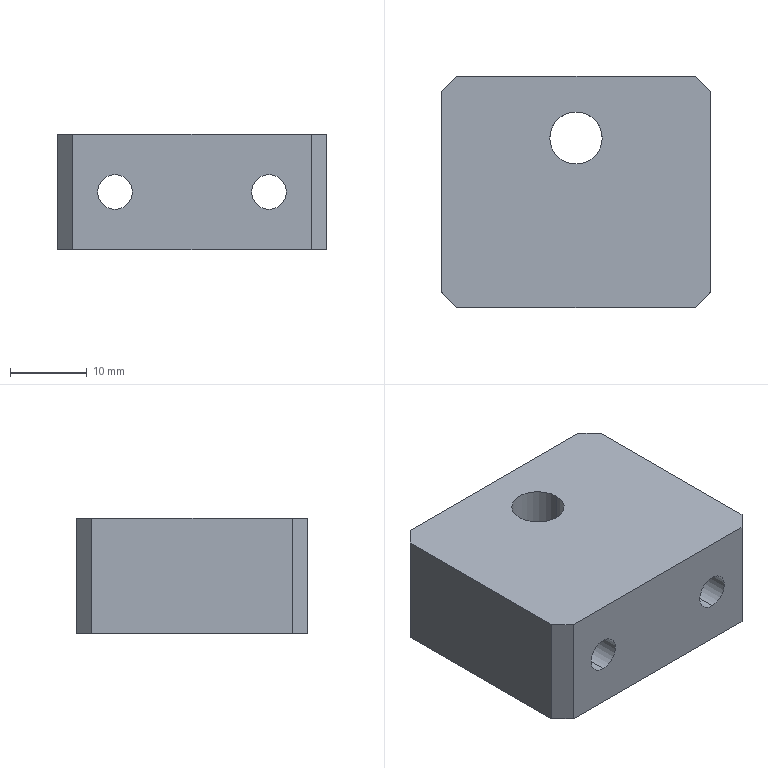Part | SolidWorks | features HoleWzd 2, Chamfer 1, Extrusion 1 | 1 solid | 22 faces | box 35 x 30 x 15 mm | volume 13829 mm3 | plane 12 | cylinder 10 | commonest cylinder face diameters 4.5 x4 8 x4 6.8 x2
STEP:
#1=CARTESIAN_POINT('',(-3.4,7.,0.));
#2=VERTEX_POINT('',#1);
#3=CARTESIAN_POINT('',(3.4,7.,0.));
#4=VERTEX_POINT('',#3);
#5=CARTESIAN_POINT('',(0.,7.,0.));
#6=DIRECTION('',(0.,0.,1.));
#7=DIRECTION('',(1.,0.,0.));
#8=AXIS2_PLACEMENT_3D('',#5,#6,#7);
#9=CIRCLE('',#8,3.4);
#10=EDGE_CURVE('',#2,#4,#9,.T.);
#11=ORIENTED_EDGE('',*,*,#10,.F.);
#12=CARTESIAN_POINT('',(-3.4,7.,15.));
#13=VERTEX_POINT('',#12);
#14=CARTESIAN_POINT('',(-3.4,7.,15.));
#15=DIRECTION('',(0.,0.,1.));
#16=VECTOR('',#15,1000.);
#17=LINE('',#14,#16);
#18=EDGE_CURVE('',#2,#13,#17,.T.);
#19=ORIENTED_EDGE('',*,*,#18,.T.);
#20=CARTESIAN_POINT('',(3.4,7.,15.));
#21=VERTEX_POINT('',#20);
#22=CARTESIAN_POINT('',(0.,7.,15.));
#23=DIRECTION('',(0.,0.,1.));
#24=DIRECTION('',(1.,0.,0.));
#25=AXIS2_PLACEMENT_3D('',#22,#23,#24);
#26=CIRCLE('',#25,3.4);
#27=EDGE_CURVE('',#13,#21,#26,.T.);
#28=ORIENTED_EDGE('',*,*,#27,.T.);
#29=CARTESIAN_POINT('',(3.4,7.,15.));
#30=DIRECTION('',(0.,0.,1.));
#31=VECTOR('',#30,1000.);
#32=LINE('',#29,#31);
#33=EDGE_CURVE('',#4,#21,#32,.T.);
#34=ORIENTED_EDGE('',*,*,#33,.F.);
#35=EDGE_LOOP('',(#11,#19,#28,#34));
#36=FACE_OUTER_BOUND('',#35,.T.);
#37=CARTESIAN_POINT('',(0.,7.,15.));
#38=DIRECTION('',(0.,0.,1.));
#39=DIRECTION('',(1.,0.,0.));
#40=AXIS2_PLACEMENT_3D('',#37,#38,#39);
#41=CYLINDRICAL_SURFACE('',#40,3.4);
#42=ADVANCED_FACE('',(#36),#41,.F.);
#43=CARTESIAN_POINT('',(-10.,10.6,3.5));
#44=VERTEX_POINT('',#43);
#45=CARTESIAN_POINT('',(-10.,10.6,11.5));
#46=VERTEX_POINT('',#45);
#47=CARTESIAN_POINT('',(-10.,10.6,7.5));
#48=DIRECTION('',(0.,1.,0.));
#49=DIRECTION('',(0.,0.,1.));
#50=AXIS2_PLACEMENT_3D('',#47,#48,#49);
#51=CIRCLE('',#50,4.);
#52=EDGE_CURVE('',#44,#46,#51,.T.);
#53=ORIENTED_EDGE('',*,*,#52,.F.);
#54=CARTESIAN_POINT('',(-10.,15.,3.5));
#55=VERTEX_POINT('',#54);
#56=CARTESIAN_POINT('',(-10.,15.,3.5));
#57=DIRECTION('',(0.,1.,0.));
#58=VECTOR('',#57,1000.);
#59=LINE('',#56,#58);
#60=EDGE_CURVE('',#44,#55,#59,.T.);
#61=ORIENTED_EDGE('',*,*,#60,.T.);
#62=CARTESIAN_POINT('',(-10.,15.,11.5));
#63=VERTEX_POINT('',#62);
#64=CARTESIAN_POINT('',(-10.,15.,7.5));
#65=DIRECTION('',(0.,1.,0.));
#66=DIRECTION('',(0.,0.,1.));
#67=AXIS2_PLACEMENT_3D('',#64,#65,#66);
#68=CIRCLE('',#67,4.);
#69=EDGE_CURVE('',#55,#63,#68,.T.);
#70=ORIENTED_EDGE('',*,*,#69,.T.);
#71=CARTESIAN_POINT('',(-10.,15.,11.5));
#72=DIRECTION('',(0.,1.,0.));
#73=VECTOR('',#72,1000.);
#74=LINE('',#71,#73);
#75=EDGE_CURVE('',#46,#63,#74,.T.);
#76=ORIENTED_EDGE('',*,*,#75,.F.);
#77=EDGE_LOOP('',(#53,#61,#70,#76));
#78=FACE_OUTER_BOUND('',#77,.T.);
#79=CARTESIAN_POINT('',(-10.,15.,7.5));
#80=DIRECTION('',(0.,1.,0.));
#81=DIRECTION('',(0.,0.,1.));
#82=AXIS2_PLACEMENT_3D('',#79,#80,#81);
#83=CYLINDRICAL_SURFACE('',#82,4.);
#84=ADVANCED_FACE('',(#78),#83,.F.);
#85=CARTESIAN_POINT('',(-10.,-15.,5.25));
#86=VERTEX_POINT('',#85);
#87=CARTESIAN_POINT('',(-10.,-15.,9.75));
#88=VERTEX_POINT('',#87);
#89=CARTESIAN_POINT('',(-10.,-15.,7.5));
#90=DIRECTION('',(0.,1.,0.));
#91=DIRECTION('',(0.,0.,1.));
#92=AXIS2_PLACEMENT_3D('',#89,#90,#91);
#93=CIRCLE('',#92,2.25);
#94=EDGE_CURVE('',#86,#88,#93,.T.);
#95=ORIENTED_EDGE('',*,*,#94,.F.);
#96=CARTESIAN_POINT('',(-10.,10.6,5.25));
#97=VERTEX_POINT('',#96);
#98=CARTESIAN_POINT('',(-10.,15.,5.25));
#99=DIRECTION('',(0.,1.,0.));
#100=VECTOR('',#99,1000.);
#101=LINE('',#98,#100);
#102=EDGE_CURVE('',#86,#97,#101,.T.);
#103=ORIENTED_EDGE('',*,*,#102,.T.);
#104=CARTESIAN_POINT('',(-10.,10.6,9.75));
#105=VERTEX_POINT('',#104);
#106=CARTESIAN_POINT('',(-10.,10.6,7.5));
#107=DIRECTION('',(0.,1.,0.));
#108=DIRECTION('',(0.,0.,1.));
#109=AXIS2_PLACEMENT_3D('',#106,#107,#108);
#110=CIRCLE('',#109,2.25);
#111=EDGE_CURVE('',#97,#105,#110,.T.);
#112=ORIENTED_EDGE('',*,*,#111,.T.);
#113=CARTESIAN_POINT('',(-10.,15.,9.75));
#114=DIRECTION('',(0.,1.,0.));
#115=VECTOR('',#114,1000.);
#116=LINE('',#113,#115);
#117=EDGE_CURVE('',#88,#105,#116,.T.);
#118=ORIENTED_EDGE('',*,*,#117,.F.);
#119=EDGE_LOOP('',(#95,#103,#112,#118));
#120=FACE_OUTER_BOUND('',#119,.T.);
#121=CARTESIAN_POINT('',(-10.,15.,7.5));
#122=DIRECTION('',(0.,1.,0.));
#123=DIRECTION('',(0.,0.,1.));
#124=AXIS2_PLACEMENT_3D('',#121,#122,#123);
#125=CYLINDRICAL_SURFACE('',#124,2.25);
#126=ADVANCED_FACE('',(#120),#125,.F.);
#127=CARTESIAN_POINT('',(10.,10.6,3.5));
#128=VERTEX_POINT('',#127);
#129=CARTESIAN_POINT('',(10.,10.6,11.5));
#130=VERTEX_POINT('',#129);
#131=CARTESIAN_POINT('',(10.,10.6,7.5));
#132=DIRECTION('',(0.,1.,0.));
#133=DIRECTION('',(0.,0.,1.));
#134=AXIS2_PLACEMENT_3D('',#131,#132,#133);
#135=CIRCLE('',#134,4.);
#136=EDGE_CURVE('',#128,#130,#135,.T.);
#137=ORIENTED_EDGE('',*,*,#136,.F.);
#138=CARTESIAN_POINT('',(10.,15.,3.5));
#139=VERTEX_POINT('',#138);
#140=CARTESIAN_POINT('',(10.,15.,3.5));
#141=DIRECTION('',(0.,1.,0.));
#142=VECTOR('',#141,1000.);
#143=LINE('',#140,#142);
#144=EDGE_CURVE('',#128,#139,#143,.T.);
#145=ORIENTED_EDGE('',*,*,#144,.T.);
#146=CARTESIAN_POINT('',(10.,15.,11.5));
#147=VERTEX_POINT('',#146);
#148=CARTESIAN_POINT('',(10.,15.,7.5));
#149=DIRECTION('',(0.,1.,0.));
#150=DIRECTION('',(0.,0.,1.));
#151=AXIS2_PLACEMENT_3D('',#148,#149,#150);
#152=CIRCLE('',#151,4.);
#153=EDGE_CURVE('',#139,#147,#152,.T.);
#154=ORIENTED_EDGE('',*,*,#153,.T.);
#155=CARTESIAN_POINT('',(10.,15.,11.5));
#156=DIRECTION('',(0.,1.,0.));
#157=VECTOR('',#156,1000.);
#158=LINE('',#155,#157);
#159=EDGE_CURVE('',#130,#147,#158,.T.);
#160=ORIENTED_EDGE('',*,*,#159,.F.);
#161=EDGE_LOOP('',(#137,#145,#154,#160));
#162=FACE_OUTER_BOUND('',#161,.T.);
#163=CARTESIAN_POINT('',(10.,15.,7.5));
#164=DIRECTION('',(0.,1.,0.));
#165=DIRECTION('',(0.,0.,1.));
#166=AXIS2_PLACEMENT_3D('',#163,#164,#165);
#167=CYLINDRICAL_SURFACE('',#166,4.);
#168=ADVANCED_FACE('',(#162),#167,.F.);
#169=CARTESIAN_POINT('',(10.,-15.,5.25));
#170=VERTEX_POINT('',#169);
#171=CARTESIAN_POINT('',(10.,-15.,9.75));
#172=VERTEX_POINT('',#171);
#173=CARTESIAN_POINT('',(10.,-15.,7.5));
#174=DIRECTION('',(0.,1.,0.));
#175=DIRECTION('',(0.,0.,1.));
#176=AXIS2_PLACEMENT_3D('',#173,#174,#175);
#177=CIRCLE('',#176,2.25);
#178=EDGE_CURVE('',#170,#172,#177,.T.);
#179=ORIENTED_EDGE('',*,*,#178,.F.);
#180=CARTESIAN_POINT('',(10.,10.6,5.25));
#181=VERTEX_POINT('',#180);
#182=CARTESIAN_POINT('',(10.,15.,5.25));
#183=DIRECTION('',(0.,1.,0.));
#184=VECTOR('',#183,1000.);
#185=LINE('',#182,#184);
#186=EDGE_CURVE('',#170,#181,#185,.T.);
#187=ORIENTED_EDGE('',*,*,#186,.T.);
#188=CARTESIAN_POINT('',(10.,10.6,9.75));
#189=VERTEX_POINT('',#188);
#190=CARTESIAN_POINT('',(10.,10.6,7.5));
#191=DIRECTION('',(0.,1.,0.));
#192=DIRECTION('',(0.,0.,1.));
#193=AXIS2_PLACEMENT_3D('',#190,#191,#192);
#194=CIRCLE('',#193,2.25);
#195=EDGE_CURVE('',#181,#189,#194,.T.);
#196=ORIENTED_EDGE('',*,*,#195,.T.);
#197=CARTESIAN_POINT('',(10.,15.,9.75));
#198=DIRECTION('',(0.,1.,0.));
#199=VECTOR('',#198,1000.);
#200=LINE('',#197,#199);
#201=EDGE_CURVE('',#172,#189,#200,.T.);
#202=ORIENTED_EDGE('',*,*,#201,.F.);
#203=EDGE_LOOP('',(#179,#187,#196,#202));
#204=FACE_OUTER_BOUND('',#203,.T.);
#205=CARTESIAN_POINT('',(10.,15.,7.5));
#206=DIRECTION('',(0.,1.,0.));
#207=DIRECTION('',(0.,0.,1.));
#208=AXIS2_PLACEMENT_3D('',#205,#206,#207);
#209=CYLINDRICAL_SURFACE('',#208,2.25);
#210=ADVANCED_FACE('',(#204),#209,.F.);
#211=CARTESIAN_POINT('',(17.5,-13.,15.));
#212=VERTEX_POINT('',#211);
#213=CARTESIAN_POINT('',(17.5,13.,15.));
#214=VERTEX_POINT('',#213);
#215=CARTESIAN_POINT('',(17.5,15.,15.));
#216=DIRECTION('',(0.,1.,0.));
#217=VECTOR('',#216,1000.);
#218=LINE('',#215,#217);
#219=EDGE_CURVE('',#212,#214,#218,.T.);
#220=ORIENTED_EDGE('',*,*,#219,.F.);
#221=CARTESIAN_POINT('',(17.5,-13.,0.));
#222=VERTEX_POINT('',#221);
#223=CARTESIAN_POINT('',(17.5,-13.,15.));
#224=DIRECTION('',(0.,0.,-1.));
#225=VECTOR('',#224,1000.);
#226=LINE('',#223,#225);
#227=EDGE_CURVE('',#212,#222,#226,.T.);
#228=ORIENTED_EDGE('',*,*,#227,.T.);
#229=CARTESIAN_POINT('',(17.5,13.,0.));
#230=VERTEX_POINT('',#229);
#231=CARTESIAN_POINT('',(17.5,15.,0.));
#232=DIRECTION('',(0.,1.,0.));
#233=VECTOR('',#232,1000.);
#234=LINE('',#231,#233);
#235=EDGE_CURVE('',#222,#230,#234,.T.);
#236=ORIENTED_EDGE('',*,*,#235,.T.);
#237=CARTESIAN_POINT('',(17.5,13.,15.));
#238=DIRECTION('',(0.,0.,1.));
#239=VECTOR('',#238,1000.);
#240=LINE('',#237,#239);
#241=EDGE_CURVE('',#230,#214,#240,.T.);
#242=ORIENTED_EDGE('',*,*,#241,.T.);
#243=EDGE_LOOP('',(#220,#228,#236,#242));
#244=FACE_OUTER_BOUND('',#243,.T.);
#245=CARTESIAN_POINT('',(17.5,15.,15.));
#246=DIRECTION('',(-1.,0.,0.));
#247=DIRECTION('',(0.,-1.,0.));
#248=AXIS2_PLACEMENT_3D('',#245,#246,#247);
#249=PLANE('',#248);
#250=ADVANCED_FACE('',(#244),#249,.F.);
#251=CARTESIAN_POINT('',(-10.,15.,7.5));
#252=DIRECTION('',(0.,1.,0.));
#253=DIRECTION('',(0.,0.,1.));
#254=AXIS2_PLACEMENT_3D('',#251,#252,#253);
#255=CIRCLE('',#254,4.);
#256=EDGE_CURVE('',#63,#55,#255,.T.);
#257=ORIENTED_EDGE('',*,*,#256,.F.);
#258=ORIENTED_EDGE('',*,*,#69,.F.);
#259=EDGE_LOOP('',(#257,#258));
#260=FACE_BOUND('',#259,.T.);
#261=CARTESIAN_POINT('',(10.,15.,7.5));
#262=DIRECTION('',(0.,1.,0.));
#263=DIRECTION('',(0.,0.,1.));
#264=AXIS2_PLACEMENT_3D('',#261,#262,#263);
#265=CIRCLE('',#264,4.);
#266=EDGE_CURVE('',#147,#139,#265,.T.);
#267=ORIENTED_EDGE('',*,*,#266,.F.);
#268=ORIENTED_EDGE('',*,*,#153,.F.);
#269=EDGE_LOOP('',(#267,#268));
#270=FACE_BOUND('',#269,.T.);
#271=CARTESIAN_POINT('',(15.5,15.,15.));
#272=VERTEX_POINT('',#271);
#273=CARTESIAN_POINT('',(-15.5,15.,15.));
#274=VERTEX_POINT('',#273);
#275=CARTESIAN_POINT('',(-17.5,15.,15.));
#276=DIRECTION('',(-1.,0.,0.));
#277=VECTOR('',#276,1000.);
#278=LINE('',#275,#277);
#279=EDGE_CURVE('',#272,#274,#278,.T.);
#280=ORIENTED_EDGE('',*,*,#279,.F.);
#281=CARTESIAN_POINT('',(15.5,15.,0.));
#282=VERTEX_POINT('',#281);
#283=CARTESIAN_POINT('',(15.5,15.,15.));
#284=DIRECTION('',(0.,0.,-1.));
#285=VECTOR('',#284,1000.);
#286=LINE('',#283,#285);
#287=EDGE_CURVE('',#272,#282,#286,.T.);
#288=ORIENTED_EDGE('',*,*,#287,.T.);
#289=CARTESIAN_POINT('',(-15.5,15.,0.));
#290=VERTEX_POINT('',#289);
#291=CARTESIAN_POINT('',(-17.5,15.,0.));
#292=DIRECTION('',(-1.,0.,0.));
#293=VECTOR('',#292,1000.);
#294=LINE('',#291,#293);
#295=EDGE_CURVE('',#282,#290,#294,.T.);
#296=ORIENTED_EDGE('',*,*,#295,.T.);
#297=CARTESIAN_POINT('',(-15.5,15.,15.));
#298=DIRECTION('',(0.,0.,1.));
#299=VECTOR('',#298,1000.);
#300=LINE('',#297,#299);
#301=EDGE_CURVE('',#290,#274,#300,.T.);
#302=ORIENTED_EDGE('',*,*,#301,.T.);
#303=EDGE_LOOP('',(#280,#288,#296,#302));
#304=FACE_OUTER_BOUND('',#303,.T.);
#305=CARTESIAN_POINT('',(-17.5,15.,15.));
#306=DIRECTION('',(0.,-1.,0.));
#307=DIRECTION('',(0.,0.,-1.));
#308=AXIS2_PLACEMENT_3D('',#305,#306,#307);
#309=PLANE('',#308);
#310=ADVANCED_FACE('',(#260,#270,#304),#309,.F.);
#311=CARTESIAN_POINT('',(-17.5,13.,0.));
#312=VERTEX_POINT('',#311);
#313=CARTESIAN_POINT('',(-17.5,-13.,0.));
#314=VERTEX_POINT('',#313);
#315=CARTESIAN_POINT('',(-17.5,15.,0.));
#316=DIRECTION('',(0.,-1.,0.));
#317=VECTOR('',#316,1000.);
#318=LINE('',#315,#317);
#319=EDGE_CURVE('',#312,#314,#318,.T.);
#320=ORIENTED_EDGE('',*,*,#319,.T.);
#321=CARTESIAN_POINT('',(-17.5,-13.,15.));
#322=VERTEX_POINT('',#321);
#323=CARTESIAN_POINT('',(-17.5,-13.,15.));
#324=DIRECTION('',(0.,0.,1.));
#325=VECTOR('',#324,1000.);
#326=LINE('',#323,#325);
#327=EDGE_CURVE('',#314,#322,#326,.T.);
#328=ORIENTED_EDGE('',*,*,#327,.T.);
#329=CARTESIAN_POINT('',(-17.5,13.,15.));
#330=VERTEX_POINT('',#329);
#331=CARTESIAN_POINT('',(-17.5,15.,15.));
#332=DIRECTION('',(0.,-1.,0.));
#333=VECTOR('',#332,1000.);
#334=LINE('',#331,#333);
#335=EDGE_CURVE('',#330,#322,#334,.T.);
#336=ORIENTED_EDGE('',*,*,#335,.F.);
#337=CARTESIAN_POINT('',(-17.5,13.,15.));
#338=DIRECTION('',(0.,0.,-1.));
#339=VECTOR('',#338,1000.);
#340=LINE('',#337,#339);
#341=EDGE_CURVE('',#330,#312,#340,.T.);
#342=ORIENTED_EDGE('',*,*,#341,.T.);
#343=EDGE_LOOP('',(#320,#328,#336,#342));
#344=FACE_OUTER_BOUND('',#343,.T.);
#345=CARTESIAN_POINT('',(-17.5,15.,15.));
#346=DIRECTION('',(1.,0.,0.));
#347=DIRECTION('',(0.,1.,0.));
#348=AXIS2_PLACEMENT_3D('',#345,#346,#347);
#349=PLANE('',#348);
#350=ADVANCED_FACE('',(#344),#349,.F.);
#351=CARTESIAN_POINT('',(-10.,-15.,7.5));
#352=DIRECTION('',(0.,1.,0.));
#353=DIRECTION('',(0.,0.,1.));
#354=AXIS2_PLACEMENT_3D('',#351,#352,#353);
#355=CIRCLE('',#354,2.25);
#356=EDGE_CURVE('',#88,#86,#355,.T.);
#357=ORIENTED_EDGE('',*,*,#356,.T.);
#358=ORIENTED_EDGE('',*,*,#94,.T.);
#359=EDGE_LOOP('',(#357,#358));
#360=FACE_BOUND('',#359,.T.);
#361=CARTESIAN_POINT('',(10.,-15.,7.5));
#362=DIRECTION('',(0.,1.,0.));
#363=DIRECTION('',(0.,0.,1.));
#364=AXIS2_PLACEMENT_3D('',#361,#362,#363);
#365=CIRCLE('',#364,2.25);
#366=EDGE_CURVE('',#172,#170,#365,.T.);
#367=ORIENTED_EDGE('',*,*,#366,.T.);
#368=ORIENTED_EDGE('',*,*,#178,.T.);
#369=EDGE_LOOP('',(#367,#368));
#370=FACE_BOUND('',#369,.T.);
#371=CARTESIAN_POINT('',(-15.5,-15.,15.));
#372=VERTEX_POINT('',#371);
#373=CARTESIAN_POINT('',(15.5,-15.,15.));
#374=VERTEX_POINT('',#373);
#375=CARTESIAN_POINT('',(-17.5,-15.,15.));
#376=DIRECTION('',(1.,0.,0.));
#377=VECTOR('',#376,1000.);
#378=LINE('',#375,#377);
#379=EDGE_CURVE('',#372,#374,#378,.T.);
#380=ORIENTED_EDGE('',*,*,#379,.F.);
#381=CARTESIAN_POINT('',(-15.5,-15.,0.));
#382=VERTEX_POINT('',#381);
#383=CARTESIAN_POINT('',(-15.5,-15.,15.));
#384=DIRECTION('',(0.,0.,-1.));
#385=VECTOR('',#384,1000.);
#386=LINE('',#383,#385);
#387=EDGE_CURVE('',#372,#382,#386,.T.);
#388=ORIENTED_EDGE('',*,*,#387,.T.);
#389=CARTESIAN_POINT('',(15.5,-15.,0.));
#390=VERTEX_POINT('',#389);
#391=CARTESIAN_POINT('',(-17.5,-15.,0.));
#392=DIRECTION('',(1.,0.,0.));
#393=VECTOR('',#392,1000.);
#394=LINE('',#391,#393);
#395=EDGE_CURVE('',#382,#390,#394,.T.);
#396=ORIENTED_EDGE('',*,*,#395,.T.);
#397=CARTESIAN_POINT('',(15.5,-15.,15.));
#398=DIRECTION('',(0.,0.,1.));
#399=VECTOR('',#398,1000.);
#400=LINE('',#397,#399);
#401=EDGE_CURVE('',#390,#374,#400,.T.);
#402=ORIENTED_EDGE('',*,*,#401,.T.);
#403=EDGE_LOOP('',(#380,#388,#396,#402));
#404=FACE_OUTER_BOUND('',#403,.T.);
#405=CARTESIAN_POINT('',(-17.5,-15.,15.));
#406=DIRECTION('',(0.,1.,0.));
#407=DIRECTION('',(0.,0.,1.));
#408=AXIS2_PLACEMENT_3D('',#405,#406,#407);
#409=PLANE('',#408);
#410=ADVANCED_FACE('',(#360,#370,#404),#409,.F.);
#411=CARTESIAN_POINT('',(0.,7.,15.));
#412=DIRECTION('',(0.,0.,1.));
#413=DIRECTION('',(1.,0.,0.));
#414=AXIS2_PLACEMENT_3D('',#411,#412,#413);
#415=CIRCLE('',#414,3.4);
#416=EDGE_CURVE('',#21,#13,#415,.T.);
#417=ORIENTED_EDGE('',*,*,#416,.F.);
#418=ORIENTED_EDGE('',*,*,#27,.F.);
#419=EDGE_LOOP('',(#417,#418));
#420=FACE_BOUND('',#419,.T.);
#421=ORIENTED_EDGE('',*,*,#335,.T.);
#422=CARTESIAN_POINT('',(-15.25,-15.25,15.));
#423=DIRECTION('',(0.7071,-0.7071,0.));
#424=VECTOR('',#423,1000.);
#425=LINE('',#422,#424);
#426=EDGE_CURVE('',#322,#372,#425,.T.);
#427=ORIENTED_EDGE('',*,*,#426,.T.);
#428=ORIENTED_EDGE('',*,*,#379,.T.);
#429=CARTESIAN_POINT('',(15.25,-15.25,15.));
#430=DIRECTION('',(0.7071,0.7071,0.));
#431=VECTOR('',#430,1000.);
#432=LINE('',#429,#431);
#433=EDGE_CURVE('',#374,#212,#432,.T.);
#434=ORIENTED_EDGE('',*,*,#433,.T.);
#435=ORIENTED_EDGE('',*,*,#219,.T.);
#436=CARTESIAN_POINT('',(15.25,15.25,15.));
#437=DIRECTION('',(-0.7071,0.7071,0.));
#438=VECTOR('',#437,1000.);
#439=LINE('',#436,#438);
#440=EDGE_CURVE('',#214,#272,#439,.T.);
#441=ORIENTED_EDGE('',*,*,#440,.T.);
#442=ORIENTED_EDGE('',*,*,#279,.T.);
#443=CARTESIAN_POINT('',(-15.25,15.25,15.));
#444=DIRECTION('',(-0.7071,-0.7071,0.));
#445=VECTOR('',#444,1000.);
#446=LINE('',#443,#445);
#447=EDGE_CURVE('',#274,#330,#446,.T.);
#448=ORIENTED_EDGE('',*,*,#447,.T.);
#449=EDGE_LOOP('',(#421,#427,#428,#434,#435,#441,#442,#448));
#450=FACE_OUTER_BOUND('',#449,.T.);
#451=CARTESIAN_POINT('',(0.,0.,15.));
#452=DIRECTION('',(0.,0.,1.));
#453=DIRECTION('',(1.,0.,0.));
#454=AXIS2_PLACEMENT_3D('',#451,#452,#453);
#455=PLANE('',#454);
#456=ADVANCED_FACE('',(#420,#450),#455,.T.);
#457=CARTESIAN_POINT('',(0.,7.,0.));
#458=DIRECTION('',(0.,0.,1.));
#459=DIRECTION('',(1.,0.,0.));
#460=AXIS2_PLACEMENT_3D('',#457,#458,#459);
#461=CIRCLE('',#460,3.4);
#462=EDGE_CURVE('',#4,#2,#461,.T.);
#463=ORIENTED_EDGE('',*,*,#462,.T.);
#464=ORIENTED_EDGE('',*,*,#10,.T.);
#465=EDGE_LOOP('',(#463,#464));
#466=FACE_BOUND('',#465,.T.);
#467=ORIENTED_EDGE('',*,*,#395,.F.);
#468=CARTESIAN_POINT('',(-15.5,-15.,0.));
#469=DIRECTION('',(-0.7071,0.7071,0.));
#470=VECTOR('',#469,1000.);
#471=LINE('',#468,#470);
#472=EDGE_CURVE('',#382,#314,#471,.T.);
#473=ORIENTED_EDGE('',*,*,#472,.T.);
#474=ORIENTED_EDGE('',*,*,#319,.F.);
#475=CARTESIAN_POINT('',(-17.5,13.,0.));
#476=DIRECTION('',(0.7071,0.7071,0.));
#477=VECTOR('',#476,1000.);
#478=LINE('',#475,#477);
#479=EDGE_CURVE('',#312,#290,#478,.T.);
#480=ORIENTED_EDGE('',*,*,#479,.T.);
#481=ORIENTED_EDGE('',*,*,#295,.F.);
#482=CARTESIAN_POINT('',(15.5,15.,0.));
#483=DIRECTION('',(0.7071,-0.7071,0.));
#484=VECTOR('',#483,1000.);
#485=LINE('',#482,#484);
#486=EDGE_CURVE('',#282,#230,#485,.T.);
#487=ORIENTED_EDGE('',*,*,#486,.T.);
#488=ORIENTED_EDGE('',*,*,#235,.F.);
#489=CARTESIAN_POINT('',(17.5,-13.,0.));
#490=DIRECTION('',(-0.7071,-0.7071,0.));
#491=VECTOR('',#490,1000.);
#492=LINE('',#489,#491);
#493=EDGE_CURVE('',#222,#390,#492,.T.);
#494=ORIENTED_EDGE('',*,*,#493,.T.);
#495=EDGE_LOOP('',(#467,#473,#474,#480,#481,#487,#488,#494));
#496=FACE_OUTER_BOUND('',#495,.T.);
#497=CARTESIAN_POINT('',(0.,0.,0.));
#498=DIRECTION('',(0.,0.,1.));
#499=DIRECTION('',(1.,0.,0.));
#500=AXIS2_PLACEMENT_3D('',#497,#498,#499);
#501=PLANE('',#500);
#502=ADVANCED_FACE('',(#466,#496),#501,.F.);
#503=ORIENTED_EDGE('',*,*,#186,.F.);
#504=ORIENTED_EDGE('',*,*,#366,.F.);
#505=ORIENTED_EDGE('',*,*,#201,.T.);
#506=CARTESIAN_POINT('',(10.,10.6,7.5));
#507=DIRECTION('',(0.,1.,0.));
#508=DIRECTION('',(0.,0.,1.));
#509=AXIS2_PLACEMENT_3D('',#506,#507,#508);
#510=CIRCLE('',#509,2.25);
#511=EDGE_CURVE('',#189,#181,#510,.T.);
#512=ORIENTED_EDGE('',*,*,#511,.T.);
#513=EDGE_LOOP('',(#503,#504,#505,#512));
#514=FACE_OUTER_BOUND('',#513,.T.);
#515=CARTESIAN_POINT('',(10.,15.,7.5));
#516=DIRECTION('',(0.,1.,0.));
#517=DIRECTION('',(0.,0.,1.));
#518=AXIS2_PLACEMENT_3D('',#515,#516,#517);
#519=CYLINDRICAL_SURFACE('',#518,2.25);
#520=ADVANCED_FACE('',(#514),#519,.F.);
#521=ORIENTED_EDGE('',*,*,#511,.F.);
#522=ORIENTED_EDGE('',*,*,#195,.F.);
#523=EDGE_LOOP('',(#521,#522));
#524=FACE_BOUND('',#523,.T.);
#525=CARTESIAN_POINT('',(10.,10.6,7.5));
#526=DIRECTION('',(0.,1.,0.));
#527=DIRECTION('',(0.,0.,1.));
#528=AXIS2_PLACEMENT_3D('',#525,#526,#527);
#529=CIRCLE('',#528,4.);
#530=EDGE_CURVE('',#130,#128,#529,.T.);
#531=ORIENTED_EDGE('',*,*,#530,.T.);
#532=ORIENTED_EDGE('',*,*,#136,.T.);
#533=EDGE_LOOP('',(#531,#532));
#534=FACE_OUTER_BOUND('',#533,.T.);
#535=CARTESIAN_POINT('',(12.25,10.6,7.5));
#536=DIRECTION('',(0.,-1.,0.));
#537=DIRECTION('',(0.,0.,-1.));
#538=AXIS2_PLACEMENT_3D('',#535,#536,#537);
#539=PLANE('',#538);
#540=ADVANCED_FACE('',(#524,#534),#539,.F.);
#541=ORIENTED_EDGE('',*,*,#144,.F.);
#542=ORIENTED_EDGE('',*,*,#530,.F.);
#543=ORIENTED_EDGE('',*,*,#159,.T.);
#544=ORIENTED_EDGE('',*,*,#266,.T.);
#545=EDGE_LOOP('',(#541,#542,#543,#544));
#546=FACE_OUTER_BOUND('',#545,.T.);
#547=CARTESIAN_POINT('',(10.,15.,7.5));
#548=DIRECTION('',(0.,1.,0.));
#549=DIRECTION('',(0.,0.,1.));
#550=AXIS2_PLACEMENT_3D('',#547,#548,#549);
#551=CYLINDRICAL_SURFACE('',#550,4.);
#552=ADVANCED_FACE('',(#546),#551,.F.);
#553=ORIENTED_EDGE('',*,*,#102,.F.);
#554=ORIENTED_EDGE('',*,*,#356,.F.);
#555=ORIENTED_EDGE('',*,*,#117,.T.);
#556=CARTESIAN_POINT('',(-10.,10.6,7.5));
#557=DIRECTION('',(0.,1.,0.));
#558=DIRECTION('',(0.,0.,1.));
#559=AXIS2_PLACEMENT_3D('',#556,#557,#558);
#560=CIRCLE('',#559,2.25);
#561=EDGE_CURVE('',#105,#97,#560,.T.);
#562=ORIENTED_EDGE('',*,*,#561,.T.);
#563=EDGE_LOOP('',(#553,#554,#555,#562));
#564=FACE_OUTER_BOUND('',#563,.T.);
#565=CARTESIAN_POINT('',(-10.,15.,7.5));
#566=DIRECTION('',(0.,1.,0.));
#567=DIRECTION('',(0.,0.,1.));
#568=AXIS2_PLACEMENT_3D('',#565,#566,#567);
#569=CYLINDRICAL_SURFACE('',#568,2.25);
#570=ADVANCED_FACE('',(#564),#569,.F.);
#571=ORIENTED_EDGE('',*,*,#561,.F.);
#572=ORIENTED_EDGE('',*,*,#111,.F.);
#573=EDGE_LOOP('',(#571,#572));
#574=FACE_BOUND('',#573,.T.);
#575=CARTESIAN_POINT('',(-10.,10.6,7.5));
#576=DIRECTION('',(0.,1.,0.));
#577=DIRECTION('',(0.,0.,1.));
#578=AXIS2_PLACEMENT_3D('',#575,#576,#577);
#579=CIRCLE('',#578,4.);
#580=EDGE_CURVE('',#46,#44,#579,.T.);
#581=ORIENTED_EDGE('',*,*,#580,.T.);
#582=ORIENTED_EDGE('',*,*,#52,.T.);
#583=EDGE_LOOP('',(#581,#582));
#584=FACE_OUTER_BOUND('',#583,.T.);
#585=CARTESIAN_POINT('',(-7.75,10.6,7.5));
#586=DIRECTION('',(0.,-1.,0.));
#587=DIRECTION('',(0.,0.,-1.));
#588=AXIS2_PLACEMENT_3D('',#585,#586,#587);
#589=PLANE('',#588);
#590=ADVANCED_FACE('',(#574,#584),#589,.F.);
#591=ORIENTED_EDGE('',*,*,#60,.F.);
#592=ORIENTED_EDGE('',*,*,#580,.F.);
#593=ORIENTED_EDGE('',*,*,#75,.T.);
#594=ORIENTED_EDGE('',*,*,#256,.T.);
#595=EDGE_LOOP('',(#591,#592,#593,#594));
#596=FACE_OUTER_BOUND('',#595,.T.);
#597=CARTESIAN_POINT('',(-10.,15.,7.5));
#598=DIRECTION('',(0.,1.,0.));
#599=DIRECTION('',(0.,0.,1.));
#600=AXIS2_PLACEMENT_3D('',#597,#598,#599);
#601=CYLINDRICAL_SURFACE('',#600,4.);
#602=ADVANCED_FACE('',(#596),#601,.F.);
#603=ORIENTED_EDGE('',*,*,#18,.F.);
#604=ORIENTED_EDGE('',*,*,#462,.F.);
#605=ORIENTED_EDGE('',*,*,#33,.T.);
#606=ORIENTED_EDGE('',*,*,#416,.T.);
#607=EDGE_LOOP('',(#603,#604,#605,#606));
#608=FACE_OUTER_BOUND('',#607,.T.);
#609=CARTESIAN_POINT('',(0.,7.,15.));
#610=DIRECTION('',(0.,0.,1.));
#611=DIRECTION('',(1.,0.,0.));
#612=AXIS2_PLACEMENT_3D('',#609,#610,#611);
#613=CYLINDRICAL_SURFACE('',#612,3.4);
#614=ADVANCED_FACE('',(#608),#613,.F.);
#615=ORIENTED_EDGE('',*,*,#426,.F.);
#616=ORIENTED_EDGE('',*,*,#327,.F.);
#617=ORIENTED_EDGE('',*,*,#472,.F.);
#618=ORIENTED_EDGE('',*,*,#387,.F.);
#619=EDGE_LOOP('',(#615,#616,#617,#618));
#620=FACE_OUTER_BOUND('',#619,.T.);
#621=CARTESIAN_POINT('',(-15.5,-15.,15.));
#622=DIRECTION('',(0.7071,0.7071,0.));
#623=DIRECTION('',(0.,0.,-1.));
#624=AXIS2_PLACEMENT_3D('',#621,#622,#623);
#625=PLANE('',#624);
#626=ADVANCED_FACE('',(#620),#625,.F.);
#627=ORIENTED_EDGE('',*,*,#433,.F.);
#628=ORIENTED_EDGE('',*,*,#401,.F.);
#629=ORIENTED_EDGE('',*,*,#493,.F.);
#630=ORIENTED_EDGE('',*,*,#227,.F.);
#631=EDGE_LOOP('',(#627,#628,#629,#630));
#632=FACE_OUTER_BOUND('',#631,.T.);
#633=CARTESIAN_POINT('',(17.5,-13.,15.));
#634=DIRECTION('',(-0.7071,0.7071,0.));
#635=DIRECTION('',(0.,0.,-1.));
#636=AXIS2_PLACEMENT_3D('',#633,#634,#635);
#637=PLANE('',#636);
#638=ADVANCED_FACE('',(#632),#637,.F.);
#639=ORIENTED_EDGE('',*,*,#440,.F.);
#640=ORIENTED_EDGE('',*,*,#241,.F.);
#641=ORIENTED_EDGE('',*,*,#486,.F.);
#642=ORIENTED_EDGE('',*,*,#287,.F.);
#643=EDGE_LOOP('',(#639,#640,#641,#642));
#644=FACE_OUTER_BOUND('',#643,.T.);
#645=CARTESIAN_POINT('',(15.5,15.,15.));
#646=DIRECTION('',(-0.7071,-0.7071,0.));
#647=DIRECTION('',(0.,0.,-1.));
#648=AXIS2_PLACEMENT_3D('',#645,#646,#647);
#649=PLANE('',#648);
#650=ADVANCED_FACE('',(#644),#649,.F.);
#651=ORIENTED_EDGE('',*,*,#447,.F.);
#652=ORIENTED_EDGE('',*,*,#301,.F.);
#653=ORIENTED_EDGE('',*,*,#479,.F.);
#654=ORIENTED_EDGE('',*,*,#341,.F.);
#655=EDGE_LOOP('',(#651,#652,#653,#654));
#656=FACE_OUTER_BOUND('',#655,.T.);
#657=CARTESIAN_POINT('',(-17.5,13.,15.));
#658=DIRECTION('',(0.7071,-0.7071,0.));
#659=DIRECTION('',(0.,0.,-1.));
#660=AXIS2_PLACEMENT_3D('',#657,#658,#659);
#661=PLANE('',#660);
#662=ADVANCED_FACE('',(#656),#661,.F.);
#663=CLOSED_SHELL('',(#42,#84,#126,#168,#210,#250,#310,#350,#410,#456,#502,#520,#540,#552,#570,#590,#602,#614,#626,#638,#650,#662));
#664=MANIFOLD_SOLID_BREP('',#663);
#665=CARTESIAN_POINT('',(0.,0.,0.));
#666=DIRECTION('',(0.,0.,1.));
#667=DIRECTION('',(1.,0.,0.));
#668=AXIS2_PLACEMENT_3D('',#665,#666,#667);
#669=(LENGTH_UNIT()NAMED_UNIT(*)SI_UNIT(.MILLI.,.METRE.));
#670=UNCERTAINTY_MEASURE_WITH_UNIT(LENGTH_MEASURE(0.00001),#669,'','');
#671=(NAMED_UNIT(*)PLANE_ANGLE_UNIT()SI_UNIT($,.RADIAN.));
#672=(NAMED_UNIT(*)SI_UNIT($,.STERADIAN.)SOLID_ANGLE_UNIT());
#673=(GEOMETRIC_REPRESENTATION_CONTEXT(3)GLOBAL_UNCERTAINTY_ASSIGNED_CONTEXT((#670))GLOBAL_UNIT_ASSIGNED_CONTEXT((#669,#671,#672))REPRESENTATION_CONTEXT('',''));
#674=ADVANCED_BREP_SHAPE_REPRESENTATION('',(#664,#668),#673);